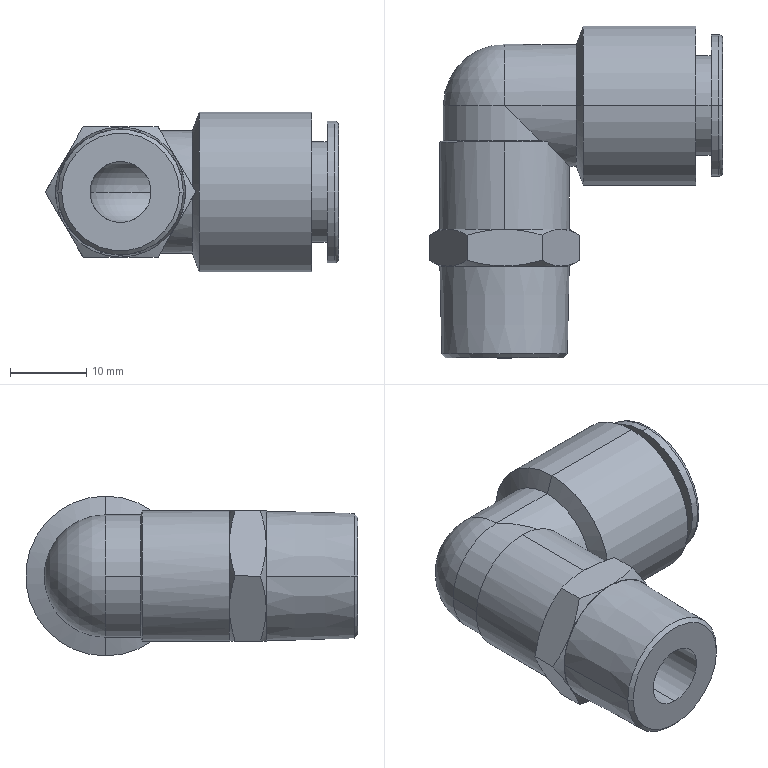Part | STEP file | KQ2L12-03S_KQ2L_12-03 | 1 solid | 56 faces | box 38.315 x 43.45 x 20.9 mm | volume 10699 mm3 | cone 21 | cylinder 16 | plane 12 | torus 6 | sphere 1 | commonest cylinder face diameters 16 x4 8 x2 12 x2 13.1 x2 17 x2 18.5 x2